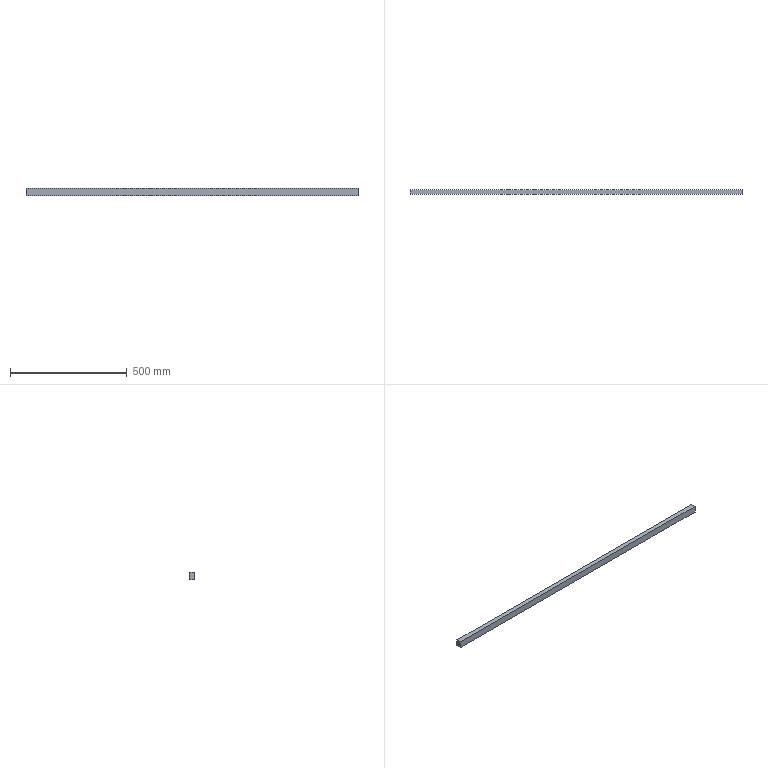Part | STEP file | Pressure plate 3 | 1 solid | 6 faces | box 1420 x 20 x 30 mm | volume 852000 mm3 | plane 6
STEP:
#1=CARTESIAN_POINT('',(710.,0.,15.));
#2=VERTEX_POINT('',#1);
#3=CARTESIAN_POINT('',(710.,0.,-15.));
#4=VERTEX_POINT('',#3);
#5=CARTESIAN_POINT('',(710.,0.,-15.));
#6=DIRECTION('',(0.,0.,-1.));
#7=VECTOR('',#6,1000.);
#8=LINE('',#5,#7);
#9=EDGE_CURVE('',#2,#4,#8,.T.);
#10=ORIENTED_EDGE('',*,*,#9,.T.);
#11=CARTESIAN_POINT('',(710.,20.,-15.));
#12=VERTEX_POINT('',#11);
#13=CARTESIAN_POINT('',(710.,20.,-15.));
#14=DIRECTION('',(0.,-1.,0.));
#15=VECTOR('',#14,1000.);
#16=LINE('',#13,#15);
#17=EDGE_CURVE('',#12,#4,#16,.T.);
#18=ORIENTED_EDGE('',*,*,#17,.F.);
#19=CARTESIAN_POINT('',(710.,20.,15.));
#20=VERTEX_POINT('',#19);
#21=CARTESIAN_POINT('',(710.,20.,-15.));
#22=DIRECTION('',(0.,0.,-1.));
#23=VECTOR('',#22,1000.);
#24=LINE('',#21,#23);
#25=EDGE_CURVE('',#20,#12,#24,.T.);
#26=ORIENTED_EDGE('',*,*,#25,.F.);
#27=CARTESIAN_POINT('',(710.,20.,15.));
#28=DIRECTION('',(0.,-1.,0.));
#29=VECTOR('',#28,1000.);
#30=LINE('',#27,#29);
#31=EDGE_CURVE('',#20,#2,#30,.T.);
#32=ORIENTED_EDGE('',*,*,#31,.T.);
#33=EDGE_LOOP('',(#10,#18,#26,#32));
#34=FACE_OUTER_BOUND('',#33,.T.);
#35=CARTESIAN_POINT('',(710.,20.,-15.));
#36=DIRECTION('',(-1.,0.,0.));
#37=DIRECTION('',(0.,0.,1.));
#38=AXIS2_PLACEMENT_3D('',#35,#36,#37);
#39=PLANE('',#38);
#40=ADVANCED_FACE('',(#34),#39,.F.);
#41=CARTESIAN_POINT('',(-710.,0.,-15.));
#42=VERTEX_POINT('',#41);
#43=CARTESIAN_POINT('',(-710.,0.,-15.));
#44=DIRECTION('',(-1.,0.,0.));
#45=VECTOR('',#44,1000.);
#46=LINE('',#43,#45);
#47=EDGE_CURVE('',#4,#42,#46,.T.);
#48=ORIENTED_EDGE('',*,*,#47,.T.);
#49=CARTESIAN_POINT('',(-710.,20.,-15.));
#50=VERTEX_POINT('',#49);
#51=CARTESIAN_POINT('',(-710.,20.,-15.));
#52=DIRECTION('',(0.,-1.,0.));
#53=VECTOR('',#52,1000.);
#54=LINE('',#51,#53);
#55=EDGE_CURVE('',#50,#42,#54,.T.);
#56=ORIENTED_EDGE('',*,*,#55,.F.);
#57=CARTESIAN_POINT('',(-710.,20.,-15.));
#58=DIRECTION('',(-1.,0.,0.));
#59=VECTOR('',#58,1000.);
#60=LINE('',#57,#59);
#61=EDGE_CURVE('',#12,#50,#60,.T.);
#62=ORIENTED_EDGE('',*,*,#61,.F.);
#63=ORIENTED_EDGE('',*,*,#17,.T.);
#64=EDGE_LOOP('',(#48,#56,#62,#63));
#65=FACE_OUTER_BOUND('',#64,.T.);
#66=CARTESIAN_POINT('',(-710.,20.,-15.));
#67=DIRECTION('',(0.,0.,1.));
#68=DIRECTION('',(1.,0.,0.));
#69=AXIS2_PLACEMENT_3D('',#66,#67,#68);
#70=PLANE('',#69);
#71=ADVANCED_FACE('',(#65),#70,.F.);
#72=CARTESIAN_POINT('',(-710.,0.,15.));
#73=VERTEX_POINT('',#72);
#74=CARTESIAN_POINT('',(-710.,0.,-15.));
#75=DIRECTION('',(0.,0.,1.));
#76=VECTOR('',#75,1000.);
#77=LINE('',#74,#76);
#78=EDGE_CURVE('',#42,#73,#77,.T.);
#79=ORIENTED_EDGE('',*,*,#78,.T.);
#80=CARTESIAN_POINT('',(-710.,20.,15.));
#81=VERTEX_POINT('',#80);
#82=CARTESIAN_POINT('',(-710.,20.,15.));
#83=DIRECTION('',(0.,-1.,0.));
#84=VECTOR('',#83,1000.);
#85=LINE('',#82,#84);
#86=EDGE_CURVE('',#81,#73,#85,.T.);
#87=ORIENTED_EDGE('',*,*,#86,.F.);
#88=CARTESIAN_POINT('',(-710.,20.,-15.));
#89=DIRECTION('',(0.,0.,1.));
#90=VECTOR('',#89,1000.);
#91=LINE('',#88,#90);
#92=EDGE_CURVE('',#50,#81,#91,.T.);
#93=ORIENTED_EDGE('',*,*,#92,.F.);
#94=ORIENTED_EDGE('',*,*,#55,.T.);
#95=EDGE_LOOP('',(#79,#87,#93,#94));
#96=FACE_OUTER_BOUND('',#95,.T.);
#97=CARTESIAN_POINT('',(-710.,20.,-15.));
#98=DIRECTION('',(1.,0.,0.));
#99=DIRECTION('',(0.,0.,-1.));
#100=AXIS2_PLACEMENT_3D('',#97,#98,#99);
#101=PLANE('',#100);
#102=ADVANCED_FACE('',(#96),#101,.F.);
#103=CARTESIAN_POINT('',(-710.,0.,15.));
#104=DIRECTION('',(1.,0.,0.));
#105=VECTOR('',#104,1000.);
#106=LINE('',#103,#105);
#107=EDGE_CURVE('',#73,#2,#106,.T.);
#108=ORIENTED_EDGE('',*,*,#107,.T.);
#109=ORIENTED_EDGE('',*,*,#31,.F.);
#110=CARTESIAN_POINT('',(-710.,20.,15.));
#111=DIRECTION('',(1.,0.,0.));
#112=VECTOR('',#111,1000.);
#113=LINE('',#110,#112);
#114=EDGE_CURVE('',#81,#20,#113,.T.);
#115=ORIENTED_EDGE('',*,*,#114,.F.);
#116=ORIENTED_EDGE('',*,*,#86,.T.);
#117=EDGE_LOOP('',(#108,#109,#115,#116));
#118=FACE_OUTER_BOUND('',#117,.T.);
#119=CARTESIAN_POINT('',(-710.,20.,15.));
#120=DIRECTION('',(0.,0.,-1.));
#121=DIRECTION('',(-1.,0.,0.));
#122=AXIS2_PLACEMENT_3D('',#119,#120,#121);
#123=PLANE('',#122);
#124=ADVANCED_FACE('',(#118),#123,.F.);
#125=ORIENTED_EDGE('',*,*,#25,.T.);
#126=ORIENTED_EDGE('',*,*,#61,.T.);
#127=ORIENTED_EDGE('',*,*,#92,.T.);
#128=ORIENTED_EDGE('',*,*,#114,.T.);
#129=EDGE_LOOP('',(#125,#126,#127,#128));
#130=FACE_OUTER_BOUND('',#129,.T.);
#131=CARTESIAN_POINT('',(0.,20.,0.));
#132=DIRECTION('',(0.,1.,0.));
#133=DIRECTION('',(0.,0.,1.));
#134=AXIS2_PLACEMENT_3D('',#131,#132,#133);
#135=PLANE('',#134);
#136=ADVANCED_FACE('',(#130),#135,.T.);
#137=ORIENTED_EDGE('',*,*,#9,.F.);
#138=ORIENTED_EDGE('',*,*,#107,.F.);
#139=ORIENTED_EDGE('',*,*,#78,.F.);
#140=ORIENTED_EDGE('',*,*,#47,.F.);
#141=EDGE_LOOP('',(#137,#138,#139,#140));
#142=FACE_OUTER_BOUND('',#141,.T.);
#143=CARTESIAN_POINT('',(0.,0.,0.));
#144=DIRECTION('',(0.,1.,0.));
#145=DIRECTION('',(0.,0.,1.));
#146=AXIS2_PLACEMENT_3D('',#143,#144,#145);
#147=PLANE('',#146);
#148=ADVANCED_FACE('',(#142),#147,.F.);
#149=CLOSED_SHELL('',(#40,#71,#102,#124,#136,#148));
#150=MANIFOLD_SOLID_BREP('',#149);
#151=CARTESIAN_POINT('',(0.,0.,0.));
#152=DIRECTION('',(0.,0.,1.));
#153=DIRECTION('',(1.,0.,0.));
#154=AXIS2_PLACEMENT_3D('',#151,#152,#153);
#155=(LENGTH_UNIT()NAMED_UNIT(*)SI_UNIT(.MILLI.,.METRE.));
#156=UNCERTAINTY_MEASURE_WITH_UNIT(LENGTH_MEASURE(0.00001),#155,'','');
#157=(NAMED_UNIT(*)PLANE_ANGLE_UNIT()SI_UNIT($,.RADIAN.));
#158=(NAMED_UNIT(*)SI_UNIT($,.STERADIAN.)SOLID_ANGLE_UNIT());
#159=(GEOMETRIC_REPRESENTATION_CONTEXT(3)GLOBAL_UNCERTAINTY_ASSIGNED_CONTEXT((#156))GLOBAL_UNIT_ASSIGNED_CONTEXT((#155,#157,#158))REPRESENTATION_CONTEXT('',''));
#160=ADVANCED_BREP_SHAPE_REPRESENTATION('',(#150,#154),#159);